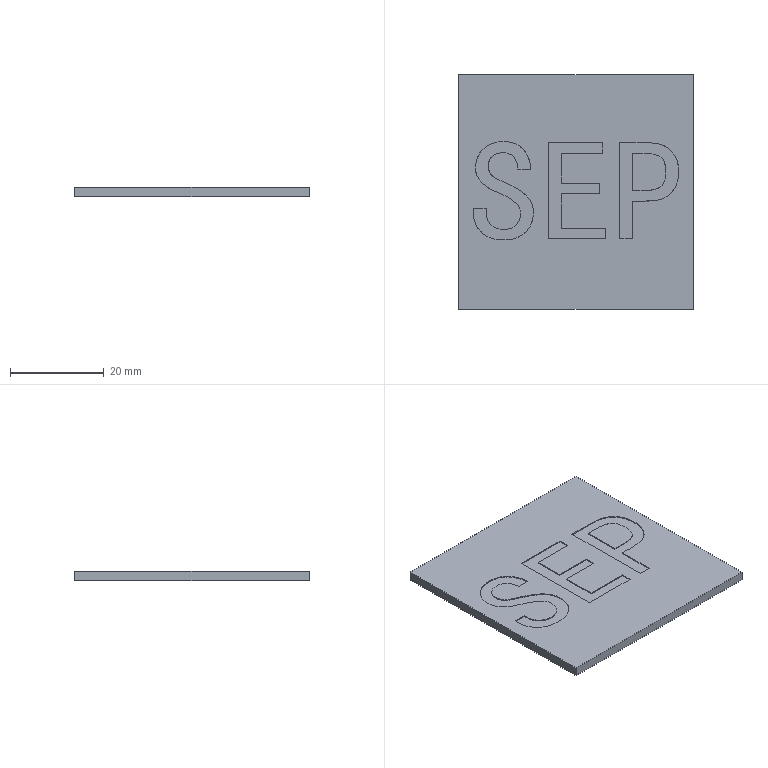Part | STEP file | lll_id1674_x_t | 1 solid | 38 faces | box 50 x 50 x 2 mm | volume 4930 mm3 | plane 28 | other 10
STEP:
#1=CARTESIAN_POINT('',(3913.931,-539.312,3.259));
#2=VERTEX_POINT('',#1);
#3=CARTESIAN_POINT('',(3918.013,-541.893,3.259));
#4=VERTEX_POINT('',#3);
#5=CARTESIAN_POINT('',(3913.931,-539.312,3.259));
#6=CARTESIAN_POINT('',(3915.691,-540.032,3.259));
#7=CARTESIAN_POINT('',(3917.052,-540.892,3.259));
#8=CARTESIAN_POINT('',(3918.013,-541.893,3.259));
#9=B_SPLINE_CURVE_WITH_KNOTS('',3,(#5,#6,#7,#8),.UNSPECIFIED.,.F.,.F.,(4,4),(0.,1.),.UNSPECIFIED.);
#10=EDGE_CURVE('',#2,#4,#9,.T.);
#11=ORIENTED_EDGE('',*,*,#10,.T.);
#12=CARTESIAN_POINT('',(3906.615,-544.587,3.259));
#13=VERTEX_POINT('',#12);
#14=CARTESIAN_POINT('',(3918.013,-541.893,3.259));
#15=CARTESIAN_POINT('',(3918.969,-542.888,3.259));
#16=CARTESIAN_POINT('',(3919.453,-544.03,3.259));
#17=CARTESIAN_POINT('',(3919.453,-547.151,3.259));
#18=CARTESIAN_POINT('',(3918.868,-548.607,3.259));
#19=CARTESIAN_POINT('',(3916.551,-550.767,3.259));
#20=CARTESIAN_POINT('',(3914.971,-551.307,3.259));
#21=CARTESIAN_POINT('',(3910.973,-551.307,3.259));
#22=CARTESIAN_POINT('',(3909.415,-550.75,3.259));
#23=CARTESIAN_POINT('',(3907.18,-548.503,3.259));
#24=CARTESIAN_POINT('',(3906.615,-547.112,3.259));
#25=CARTESIAN_POINT('',(3906.615,-545.149,3.259));
#26=CARTESIAN_POINT('',(3906.615,-544.868,3.259));
#27=CARTESIAN_POINT('',(3906.615,-544.587,3.259));
#28=B_SPLINE_CURVE_WITH_KNOTS('',3,(#14,#15,#16,#17,#18,#19,#20,#21,#22,#23,#24,#25,#26,#27),.UNSPECIFIED.,.F.,.F.,(4,2,2,2,2,2,4),(0.,0.1423,0.348,0.5536,0.7599,0.9656,1.),.UNSPECIFIED.);
#29=EDGE_CURVE('',#4,#13,#28,.T.);
#30=ORIENTED_EDGE('',*,*,#29,.T.);
#31=CARTESIAN_POINT('',(3909.376,-544.587,3.259));
#32=VERTEX_POINT('',#31);
#33=CARTESIAN_POINT('',(3907.995,-544.587,3.259));
#34=DIRECTION('',(1.,0.,0.));
#35=VECTOR('',#34,1.);
#36=LINE('',#33,#35);
#37=EDGE_CURVE('',#13,#32,#36,.T.);
#38=ORIENTED_EDGE('',*,*,#37,.T.);
#39=CARTESIAN_POINT('',(3912.491,-541.471,3.259));
#40=VERTEX_POINT('',#39);
#41=CARTESIAN_POINT('',(3909.376,-544.587,3.259));
#42=CARTESIAN_POINT('',(3909.376,-544.827,3.259));
#43=CARTESIAN_POINT('',(3909.376,-545.067,3.259));
#44=CARTESIAN_POINT('',(3909.376,-546.51,3.259));
#45=CARTESIAN_POINT('',(3909.736,-547.427,3.259));
#46=CARTESIAN_POINT('',(3911.175,-548.709,3.259));
#47=CARTESIAN_POINT('',(3912.013,-549.029,3.259));
#48=CARTESIAN_POINT('',(3914.251,-549.029,3.259));
#49=CARTESIAN_POINT('',(3915.19,-548.686,3.259));
#50=CARTESIAN_POINT('',(3916.391,-547.328,3.259));
#51=CARTESIAN_POINT('',(3916.692,-546.51,3.259));
#52=CARTESIAN_POINT('',(3916.692,-544.75,3.259));
#53=CARTESIAN_POINT('',(3916.332,-544.008,3.259));
#54=CARTESIAN_POINT('',(3914.889,-542.655,3.259));
#55=CARTESIAN_POINT('',(3913.852,-542.028,3.259));
#56=CARTESIAN_POINT('',(3912.491,-541.471,3.259));
#57=B_SPLINE_CURVE_WITH_KNOTS('',3,(#41,#42,#43,#44,#45,#46,#47,#48,#49,#50,#51,#52,#53,#54,#55,#56),.UNSPECIFIED.,.F.,.F.,(4,2,2,2,2,2,2,4),(0.,0.02829,0.1702,0.3121,0.5005,0.688,0.8437,1.),.UNSPECIFIED.);
#58=EDGE_CURVE('',#32,#40,#57,.T.);
#59=ORIENTED_EDGE('',*,*,#58,.T.);
#60=CARTESIAN_POINT('',(3918.851,-536.191,3.259));
#61=VERTEX_POINT('',#60);
#62=CARTESIAN_POINT('',(3912.491,-541.471,3.259));
#63=CARTESIAN_POINT('',(3910.573,-540.752,3.259));
#64=CARTESIAN_POINT('',(3909.196,-539.953,3.259));
#65=CARTESIAN_POINT('',(3907.514,-538.193,3.259));
#66=CARTESIAN_POINT('',(3907.092,-537.152,3.259));
#67=CARTESIAN_POINT('',(3907.092,-534.273,3.259));
#68=CARTESIAN_POINT('',(3907.672,-532.912,3.259));
#69=CARTESIAN_POINT('',(3909.997,-530.835,3.259));
#70=CARTESIAN_POINT('',(3911.372,-530.314,3.259));
#71=CARTESIAN_POINT('',(3915.05,-530.314,3.259));
#72=CARTESIAN_POINT('',(3916.551,-530.933,3.259));
#73=CARTESIAN_POINT('',(3918.391,-533.412,3.259));
#74=CARTESIAN_POINT('',(3918.851,-534.751,3.259));
#75=CARTESIAN_POINT('',(3918.851,-536.191,3.259));
#76=B_SPLINE_CURVE_WITH_KNOTS('',3,(#62,#63,#64,#65,#66,#67,#68,#69,#70,#71,#72,#73,#74,#75),.UNSPECIFIED.,.F.,.F.,(4,2,2,2,2,2,4),(0.,0.1195,0.2381,0.4047,0.5709,0.786,1.),.UNSPECIFIED.);
#77=EDGE_CURVE('',#40,#61,#76,.T.);
#78=ORIENTED_EDGE('',*,*,#77,.T.);
#79=CARTESIAN_POINT('',(3916.09,-536.191,3.259));
#80=VERTEX_POINT('',#79);
#81=CARTESIAN_POINT('',(3917.471,-536.191,3.259));
#82=DIRECTION('',(-1.,0.,0.));
#83=VECTOR('',#82,1.);
#84=LINE('',#81,#83);
#85=EDGE_CURVE('',#61,#80,#84,.T.);
#86=ORIENTED_EDGE('',*,*,#85,.T.);
#87=CARTESIAN_POINT('',(3910.692,-533.492,3.259));
#88=VERTEX_POINT('',#87);
#89=CARTESIAN_POINT('',(3916.09,-536.191,3.259));
#90=CARTESIAN_POINT('',(3916.169,-535.314,3.259));
#91=CARTESIAN_POINT('',(3915.933,-534.515,3.259));
#92=CARTESIAN_POINT('',(3914.81,-533.078,3.259));
#93=CARTESIAN_POINT('',(3914.009,-532.716,3.259));
#94=CARTESIAN_POINT('',(3912.013,-532.716,3.259));
#95=CARTESIAN_POINT('',(3911.254,-532.974,3.259));
#96=CARTESIAN_POINT('',(3910.692,-533.492,3.259));
#97=B_SPLINE_CURVE_WITH_KNOTS('',3,(#89,#90,#91,#92,#93,#94,#95,#96),.UNSPECIFIED.,.F.,.F.,(4,2,2,4),(0.,0.3422,0.6832,1.),.UNSPECIFIED.);
#98=EDGE_CURVE('',#80,#88,#97,.T.);
#99=ORIENTED_EDGE('',*,*,#98,.T.);
#100=CARTESIAN_POINT('',(3910.692,-533.492,3.259));
#101=CARTESIAN_POINT('',(3910.135,-534.015,3.259));
#102=CARTESIAN_POINT('',(3909.854,-534.712,3.259));
#103=CARTESIAN_POINT('',(3909.854,-536.315,3.259));
#104=CARTESIAN_POINT('',(3910.073,-536.933,3.259));
#105=CARTESIAN_POINT('',(3910.955,-537.974,3.259));
#106=CARTESIAN_POINT('',(3912.092,-538.592,3.259));
#107=CARTESIAN_POINT('',(3913.931,-539.312,3.259));
#108=B_SPLINE_CURVE_WITH_KNOTS('',3,(#100,#101,#102,#103,#104,#105,#106,#107),.UNSPECIFIED.,.F.,.F.,(4,2,2,4),(0.,0.3788,0.6876,1.),.UNSPECIFIED.);
#109=EDGE_CURVE('',#88,#2,#108,.T.);
#110=ORIENTED_EDGE('',*,*,#109,.T.);
#111=EDGE_LOOP('',(#11,#30,#38,#59,#78,#86,#99,#110));
#112=FACE_BOUND('',#111,.T.);
#113=CARTESIAN_POINT('',(3953.509,-566.065,3.259));
#114=VERTEX_POINT('',#113);
#115=CARTESIAN_POINT('',(3903.509,-566.065,3.259));
#116=VERTEX_POINT('',#115);
#117=CARTESIAN_POINT('',(4003.509,-566.065,3.259));
#118=DIRECTION('',(-1.,0.,0.));
#119=VECTOR('',#118,1.);
#120=LINE('',#117,#119);
#121=EDGE_CURVE('',#114,#116,#120,.T.);
#122=ORIENTED_EDGE('',*,*,#121,.F.);
#123=CARTESIAN_POINT('',(3953.509,-516.065,3.259));
#124=VERTEX_POINT('',#123);
#125=CARTESIAN_POINT('',(3953.509,-466.065,3.259));
#126=DIRECTION('',(0.,-1.,0.));
#127=VECTOR('',#126,1.);
#128=LINE('',#125,#127);
#129=EDGE_CURVE('',#124,#114,#128,.T.);
#130=ORIENTED_EDGE('',*,*,#129,.F.);
#131=CARTESIAN_POINT('',(3903.509,-516.065,3.259));
#132=VERTEX_POINT('',#131);
#133=CARTESIAN_POINT('',(4003.509,-516.065,3.259));
#134=DIRECTION('',(-1.,0.,0.));
#135=VECTOR('',#134,1.);
#136=LINE('',#133,#135);
#137=EDGE_CURVE('',#124,#132,#136,.T.);
#138=ORIENTED_EDGE('',*,*,#137,.T.);
#139=CARTESIAN_POINT('',(3903.509,-466.065,3.259));
#140=DIRECTION('',(0.,1.,0.));
#141=VECTOR('',#140,1.);
#142=LINE('',#139,#141);
#143=EDGE_CURVE('',#116,#132,#142,.T.);
#144=ORIENTED_EDGE('',*,*,#143,.F.);
#145=EDGE_LOOP('',(#122,#130,#138,#144));
#146=FACE_BOUND('',#145,.T.);
#147=CARTESIAN_POINT('',(3925.329,-548.787,3.259));
#148=VERTEX_POINT('',#147);
#149=CARTESIAN_POINT('',(3934.811,-548.787,3.259));
#150=VERTEX_POINT('',#149);
#151=CARTESIAN_POINT('',(3930.07,-548.787,3.259));
#152=DIRECTION('',(1.,0.,0.));
#153=VECTOR('',#152,1.);
#154=LINE('',#151,#153);
#155=EDGE_CURVE('',#148,#150,#154,.T.);
#156=ORIENTED_EDGE('',*,*,#155,.T.);
#157=CARTESIAN_POINT('',(3934.811,-551.065,3.259));
#158=VERTEX_POINT('',#157);
#159=CARTESIAN_POINT('',(3934.811,-549.926,3.259));
#160=DIRECTION('',(0.,-1.,0.));
#161=VECTOR('',#160,1.);
#162=LINE('',#159,#161);
#163=EDGE_CURVE('',#150,#158,#162,.T.);
#164=ORIENTED_EDGE('',*,*,#163,.T.);
#165=CARTESIAN_POINT('',(3922.574,-551.065,3.259));
#166=VERTEX_POINT('',#165);
#167=CARTESIAN_POINT('',(3928.692,-551.065,3.259));
#168=DIRECTION('',(-1.,0.,0.));
#169=VECTOR('',#168,1.);
#170=LINE('',#167,#169);
#171=EDGE_CURVE('',#158,#166,#170,.T.);
#172=ORIENTED_EDGE('',*,*,#171,.T.);
#173=CARTESIAN_POINT('',(3922.574,-530.556,3.259));
#174=VERTEX_POINT('',#173);
#175=CARTESIAN_POINT('',(3922.574,-540.811,3.259));
#176=DIRECTION('',(0.,1.,0.));
#177=VECTOR('',#176,1.);
#178=LINE('',#175,#177);
#179=EDGE_CURVE('',#166,#174,#178,.T.);
#180=ORIENTED_EDGE('',*,*,#179,.T.);
#181=CARTESIAN_POINT('',(3934.209,-530.556,3.259));
#182=VERTEX_POINT('',#181);
#183=CARTESIAN_POINT('',(3928.391,-530.556,3.259));
#184=DIRECTION('',(1.,0.,0.));
#185=VECTOR('',#184,1.);
#186=LINE('',#183,#185);
#187=EDGE_CURVE('',#174,#182,#186,.T.);
#188=ORIENTED_EDGE('',*,*,#187,.T.);
#189=CARTESIAN_POINT('',(3934.209,-532.834,3.259));
#190=VERTEX_POINT('',#189);
#191=CARTESIAN_POINT('',(3934.209,-531.695,3.259));
#192=DIRECTION('',(0.,-1.,0.));
#193=VECTOR('',#192,1.);
#194=LINE('',#191,#193);
#195=EDGE_CURVE('',#182,#190,#194,.T.);
#196=ORIENTED_EDGE('',*,*,#195,.T.);
#197=CARTESIAN_POINT('',(3925.329,-532.834,3.259));
#198=VERTEX_POINT('',#197);
#199=CARTESIAN_POINT('',(3929.769,-532.834,3.259));
#200=DIRECTION('',(-1.,0.,0.));
#201=VECTOR('',#200,1.);
#202=LINE('',#199,#201);
#203=EDGE_CURVE('',#190,#198,#202,.T.);
#204=ORIENTED_EDGE('',*,*,#203,.T.);
#205=CARTESIAN_POINT('',(3925.329,-539.194,3.259));
#206=VERTEX_POINT('',#205);
#207=CARTESIAN_POINT('',(3925.329,-536.014,3.259));
#208=DIRECTION('',(0.,-1.,0.));
#209=VECTOR('',#208,1.);
#210=LINE('',#207,#209);
#211=EDGE_CURVE('',#198,#206,#210,.T.);
#212=ORIENTED_EDGE('',*,*,#211,.T.);
#213=CARTESIAN_POINT('',(3933.489,-539.194,3.259));
#214=VERTEX_POINT('',#213);
#215=CARTESIAN_POINT('',(3929.409,-539.194,3.259));
#216=DIRECTION('',(1.,0.,0.));
#217=VECTOR('',#216,1.);
#218=LINE('',#215,#217);
#219=EDGE_CURVE('',#206,#214,#218,.T.);
#220=ORIENTED_EDGE('',*,*,#219,.T.);
#221=CARTESIAN_POINT('',(3933.489,-541.471,3.259));
#222=VERTEX_POINT('',#221);
#223=CARTESIAN_POINT('',(3933.489,-540.333,3.259));
#224=DIRECTION('',(0.,-1.,0.));
#225=VECTOR('',#224,1.);
#226=LINE('',#223,#225);
#227=EDGE_CURVE('',#214,#222,#226,.T.);
#228=ORIENTED_EDGE('',*,*,#227,.T.);
#229=CARTESIAN_POINT('',(3925.329,-541.471,3.259));
#230=VERTEX_POINT('',#229);
#231=CARTESIAN_POINT('',(3929.409,-541.471,3.259));
#232=DIRECTION('',(-1.,0.,0.));
#233=VECTOR('',#232,1.);
#234=LINE('',#231,#233);
#235=EDGE_CURVE('',#222,#230,#234,.T.);
#236=ORIENTED_EDGE('',*,*,#235,.T.);
#237=CARTESIAN_POINT('',(3925.329,-545.129,3.259));
#238=DIRECTION('',(0.,-1.,0.));
#239=VECTOR('',#238,1.);
#240=LINE('',#237,#239);
#241=EDGE_CURVE('',#230,#148,#240,.T.);
#242=ORIENTED_EDGE('',*,*,#241,.T.);
#243=EDGE_LOOP('',(#156,#164,#172,#180,#188,#196,#204,#212,#220,#228,#236,#242));
#244=FACE_BOUND('',#243,.T.);
#245=CARTESIAN_POINT('',(3937.808,-530.556,3.259));
#246=VERTEX_POINT('',#245);
#247=CARTESIAN_POINT('',(3948.729,-532.232,3.259));
#248=VERTEX_POINT('',#247);
#249=CARTESIAN_POINT('',(3937.808,-530.556,3.259));
#250=CARTESIAN_POINT('',(3939.889,-530.556,3.259));
#251=CARTESIAN_POINT('',(3941.969,-530.556,3.259));
#252=CARTESIAN_POINT('',(3946.046,-530.556,3.259));
#253=CARTESIAN_POINT('',(3947.604,-531.113,3.259));
#254=CARTESIAN_POINT('',(3948.729,-532.232,3.259));
#255=B_SPLINE_CURVE_WITH_KNOTS('',3,(#249,#250,#251,#252,#253,#254),.UNSPECIFIED.,.F.,.F.,(4,2,4),(0.,0.5103,1.),.UNSPECIFIED.);
#256=EDGE_CURVE('',#246,#248,#255,.T.);
#257=ORIENTED_EDGE('',*,*,#256,.T.);
#258=CARTESIAN_POINT('',(3940.569,-543.029,3.259));
#259=VERTEX_POINT('',#258);
#260=CARTESIAN_POINT('',(3948.729,-532.232,3.259));
#261=CARTESIAN_POINT('',(3949.848,-533.351,3.259));
#262=CARTESIAN_POINT('',(3950.404,-534.875,3.259));
#263=CARTESIAN_POINT('',(3950.404,-538.71,3.259));
#264=CARTESIAN_POINT('',(3949.848,-540.229,3.259));
#265=CARTESIAN_POINT('',(3947.61,-542.478,3.259));
#266=CARTESIAN_POINT('',(3946.046,-543.029,3.259));
#267=CARTESIAN_POINT('',(3942.89,-543.029,3.259));
#268=CARTESIAN_POINT('',(3941.729,-543.029,3.259));
#269=CARTESIAN_POINT('',(3940.569,-543.029,3.259));
#270=B_SPLINE_CURVE_WITH_KNOTS('',3,(#260,#261,#262,#263,#264,#265,#266,#267,#268,#269),.UNSPECIFIED.,.F.,.F.,(4,2,2,2,4),(0.,0.2792,0.5585,0.8377,1.),.UNSPECIFIED.);
#271=EDGE_CURVE('',#248,#259,#270,.T.);
#272=ORIENTED_EDGE('',*,*,#271,.T.);
#273=CARTESIAN_POINT('',(3940.569,-551.065,3.259));
#274=VERTEX_POINT('',#273);
#275=CARTESIAN_POINT('',(3940.569,-547.047,3.259));
#276=DIRECTION('',(0.,-1.,0.));
#277=VECTOR('',#276,1.);
#278=LINE('',#275,#277);
#279=EDGE_CURVE('',#259,#274,#278,.T.);
#280=ORIENTED_EDGE('',*,*,#279,.T.);
#281=CARTESIAN_POINT('',(3937.808,-551.065,3.259));
#282=VERTEX_POINT('',#281);
#283=CARTESIAN_POINT('',(3939.188,-551.065,3.259));
#284=DIRECTION('',(-1.,0.,0.));
#285=VECTOR('',#284,1.);
#286=LINE('',#283,#285);
#287=EDGE_CURVE('',#274,#282,#286,.T.);
#288=ORIENTED_EDGE('',*,*,#287,.T.);
#289=CARTESIAN_POINT('',(3937.808,-540.811,3.259));
#290=DIRECTION('',(0.,1.,0.));
#291=VECTOR('',#290,1.);
#292=LINE('',#289,#291);
#293=EDGE_CURVE('',#282,#246,#292,.T.);
#294=ORIENTED_EDGE('',*,*,#293,.T.);
#295=EDGE_LOOP('',(#257,#272,#280,#288,#294));
#296=FACE_BOUND('',#295,.T.);
#297=CARTESIAN_POINT('',(4003.509,-466.065,3.259));
#298=DIRECTION('',(0.,0.,1.));
#299=DIRECTION('',(1.,0.,0.));
#300=AXIS2_PLACEMENT_3D('',#297,#298,#299);
#301=PLANE('',#300);
#302=ADVANCED_FACE('',(#112,#146,#244,#296),#301,.T.);
#303=CARTESIAN_POINT('',(3953.509,-566.065,1.259));
#304=VERTEX_POINT('',#303);
#305=CARTESIAN_POINT('',(3953.509,-566.065,179.534));
#306=DIRECTION('',(0.,0.,1.));
#307=VECTOR('',#306,1.);
#308=LINE('',#305,#307);
#309=EDGE_CURVE('',#304,#114,#308,.T.);
#310=ORIENTED_EDGE('',*,*,#309,.F.);
#311=CARTESIAN_POINT('',(3953.509,-516.065,1.259));
#312=VERTEX_POINT('',#311);
#313=CARTESIAN_POINT('',(3953.509,-466.065,1.259));
#314=DIRECTION('',(0.,-1.,0.));
#315=VECTOR('',#314,1.);
#316=LINE('',#313,#315);
#317=EDGE_CURVE('',#312,#304,#316,.T.);
#318=ORIENTED_EDGE('',*,*,#317,.F.);
#319=CARTESIAN_POINT('',(3953.509,-516.065,2.109));
#320=DIRECTION('',(0.,0.,-1.));
#321=VECTOR('',#320,1.);
#322=LINE('',#319,#321);
#323=EDGE_CURVE('',#124,#312,#322,.T.);
#324=ORIENTED_EDGE('',*,*,#323,.F.);
#325=ORIENTED_EDGE('',*,*,#129,.T.);
#326=EDGE_LOOP('',(#310,#318,#324,#325));
#327=FACE_OUTER_BOUND('',#326,.T.);
#328=CARTESIAN_POINT('',(3953.509,-541.065,2.259));
#329=DIRECTION('',(1.,0.,0.));
#330=DIRECTION('',(0.,0.,-1.));
#331=AXIS2_PLACEMENT_3D('',#328,#329,#330);
#332=PLANE('',#331);
#333=ADVANCED_FACE('',(#327),#332,.T.);
#334=CARTESIAN_POINT('',(3903.509,-516.065,1.259));
#335=VERTEX_POINT('',#334);
#336=CARTESIAN_POINT('',(3903.509,-516.065,2.109));
#337=DIRECTION('',(0.,0.,1.));
#338=VECTOR('',#337,1.);
#339=LINE('',#336,#338);
#340=EDGE_CURVE('',#335,#132,#339,.T.);
#341=ORIENTED_EDGE('',*,*,#340,.F.);
#342=CARTESIAN_POINT('',(3903.509,-566.065,1.259));
#343=VERTEX_POINT('',#342);
#344=CARTESIAN_POINT('',(3903.509,-466.065,1.259));
#345=DIRECTION('',(0.,-1.,0.));
#346=VECTOR('',#345,1.);
#347=LINE('',#344,#346);
#348=EDGE_CURVE('',#335,#343,#347,.T.);
#349=ORIENTED_EDGE('',*,*,#348,.T.);
#350=CARTESIAN_POINT('',(3903.509,-566.065,179.534));
#351=DIRECTION('',(0.,0.,1.));
#352=VECTOR('',#351,1.);
#353=LINE('',#350,#352);
#354=EDGE_CURVE('',#343,#116,#353,.T.);
#355=ORIENTED_EDGE('',*,*,#354,.T.);
#356=ORIENTED_EDGE('',*,*,#143,.T.);
#357=EDGE_LOOP('',(#341,#349,#355,#356));
#358=FACE_OUTER_BOUND('',#357,.T.);
#359=CARTESIAN_POINT('',(3903.509,-516.065,2.109));
#360=DIRECTION('',(1.,0.,0.));
#361=DIRECTION('',(0.,0.,-1.));
#362=AXIS2_PLACEMENT_3D('',#359,#360,#361);
#363=PLANE('',#362);
#364=ADVANCED_FACE('',(#358),#363,.F.);
#365=ORIENTED_EDGE('',*,*,#137,.F.);
#366=ORIENTED_EDGE('',*,*,#323,.T.);
#367=CARTESIAN_POINT('',(2443.509,-516.065,1.259));
#368=DIRECTION('',(1.,0.,0.));
#369=VECTOR('',#368,1.);
#370=LINE('',#367,#369);
#371=EDGE_CURVE('',#335,#312,#370,.T.);
#372=ORIENTED_EDGE('',*,*,#371,.F.);
#373=ORIENTED_EDGE('',*,*,#340,.T.);
#374=EDGE_LOOP('',(#365,#366,#372,#373));
#375=FACE_OUTER_BOUND('',#374,.T.);
#376=CARTESIAN_POINT('',(3953.509,-516.065,2.109));
#377=DIRECTION('',(0.,1.,0.));
#378=DIRECTION('',(0.,0.,1.));
#379=AXIS2_PLACEMENT_3D('',#376,#377,#378);
#380=PLANE('',#379);
#381=ADVANCED_FACE('',(#375),#380,.T.);
#382=CARTESIAN_POINT('',(-3312.62,-566.065,1.259));
#383=DIRECTION('',(1.,0.,0.));
#384=VECTOR('',#383,1.);
#385=LINE('',#382,#384);
#386=EDGE_CURVE('',#343,#304,#385,.T.);
#387=ORIENTED_EDGE('',*,*,#386,.T.);
#388=ORIENTED_EDGE('',*,*,#309,.T.);
#389=ORIENTED_EDGE('',*,*,#121,.T.);
#390=ORIENTED_EDGE('',*,*,#354,.F.);
#391=EDGE_LOOP('',(#387,#388,#389,#390));
#392=FACE_OUTER_BOUND('',#391,.T.);
#393=CARTESIAN_POINT('',(-3312.62,-566.065,179.534));
#394=DIRECTION('',(0.,-1.,0.));
#395=DIRECTION('',(0.,0.,-1.));
#396=AXIS2_PLACEMENT_3D('',#393,#394,#395);
#397=PLANE('',#396);
#398=ADVANCED_FACE('',(#392),#397,.T.);
#399=ORIENTED_EDGE('',*,*,#371,.T.);
#400=ORIENTED_EDGE('',*,*,#317,.T.);
#401=ORIENTED_EDGE('',*,*,#386,.F.);
#402=ORIENTED_EDGE('',*,*,#348,.F.);
#403=EDGE_LOOP('',(#399,#400,#401,#402));
#404=FACE_OUTER_BOUND('',#403,.T.);
#405=CARTESIAN_POINT('',(2443.509,-466.065,1.259));
#406=DIRECTION('',(0.,0.,-1.));
#407=DIRECTION('',(-1.,0.,0.));
#408=AXIS2_PLACEMENT_3D('',#405,#406,#407);
#409=PLANE('',#408);
#410=ADVANCED_FACE('',(#404),#409,.T.);
#411=ORIENTED_EDGE('',*,*,#163,.F.);
#412=CARTESIAN_POINT('',(3934.811,-548.787,3.059));
#413=VERTEX_POINT('',#412);
#414=CARTESIAN_POINT('',(3934.811,-548.787,3.059));
#415=DIRECTION('',(0.,0.,-1.));
#416=VECTOR('',#415,1.);
#417=LINE('',#414,#416);
#418=EDGE_CURVE('',#150,#413,#417,.T.);
#419=ORIENTED_EDGE('',*,*,#418,.T.);
#420=CARTESIAN_POINT('',(3934.811,-551.065,3.059));
#421=VERTEX_POINT('',#420);
#422=CARTESIAN_POINT('',(3934.811,-549.926,3.059));
#423=DIRECTION('',(0.,1.,0.));
#424=VECTOR('',#423,1.);
#425=LINE('',#422,#424);
#426=EDGE_CURVE('',#421,#413,#425,.T.);
#427=ORIENTED_EDGE('',*,*,#426,.F.);
#428=CARTESIAN_POINT('',(3934.811,-551.065,3.059));
#429=DIRECTION('',(0.,0.,-1.));
#430=VECTOR('',#429,1.);
#431=LINE('',#428,#430);
#432=EDGE_CURVE('',#158,#421,#431,.T.);
#433=ORIENTED_EDGE('',*,*,#432,.F.);
#434=EDGE_LOOP('',(#411,#419,#427,#433));
#435=FACE_OUTER_BOUND('',#434,.T.);
#436=CARTESIAN_POINT('',(3934.811,-548.787,3.059));
#437=DIRECTION('',(-1.,0.,0.));
#438=DIRECTION('',(0.,0.,1.));
#439=AXIS2_PLACEMENT_3D('',#436,#437,#438);
#440=PLANE('',#439);
#441=ADVANCED_FACE('',(#435),#440,.T.);
#442=ORIENTED_EDGE('',*,*,#171,.F.);
#443=ORIENTED_EDGE('',*,*,#432,.T.);
#444=CARTESIAN_POINT('',(3922.574,-551.065,3.059));
#445=VERTEX_POINT('',#444);
#446=CARTESIAN_POINT('',(3928.692,-551.065,3.059));
#447=DIRECTION('',(1.,0.,0.));
#448=VECTOR('',#447,1.);
#449=LINE('',#446,#448);
#450=EDGE_CURVE('',#445,#421,#449,.T.);
#451=ORIENTED_EDGE('',*,*,#450,.F.);
#452=CARTESIAN_POINT('',(3922.574,-551.065,3.059));
#453=DIRECTION('',(0.,0.,-1.));
#454=VECTOR('',#453,1.);
#455=LINE('',#452,#454);
#456=EDGE_CURVE('',#166,#445,#455,.T.);
#457=ORIENTED_EDGE('',*,*,#456,.F.);
#458=EDGE_LOOP('',(#442,#443,#451,#457));
#459=FACE_OUTER_BOUND('',#458,.T.);
#460=CARTESIAN_POINT('',(3934.811,-551.065,3.059));
#461=DIRECTION('',(0.,1.,0.));
#462=DIRECTION('',(0.,0.,1.));
#463=AXIS2_PLACEMENT_3D('',#460,#461,#462);
#464=PLANE('',#463);
#465=ADVANCED_FACE('',(#459),#464,.T.);
#466=ORIENTED_EDGE('',*,*,#179,.F.);
#467=ORIENTED_EDGE('',*,*,#456,.T.);
#468=CARTESIAN_POINT('',(3922.574,-530.556,3.059));
#469=VERTEX_POINT('',#468);
#470=CARTESIAN_POINT('',(3922.574,-540.811,3.059));
#471=DIRECTION('',(0.,-1.,0.));
#472=VECTOR('',#471,1.);
#473=LINE('',#470,#472);
#474=EDGE_CURVE('',#469,#445,#473,.T.);
#475=ORIENTED_EDGE('',*,*,#474,.F.);
#476=CARTESIAN_POINT('',(3922.574,-530.556,3.059));
#477=DIRECTION('',(0.,0.,-1.));
#478=VECTOR('',#477,1.);
#479=LINE('',#476,#478);
#480=EDGE_CURVE('',#174,#469,#479,.T.);
#481=ORIENTED_EDGE('',*,*,#480,.F.);
#482=EDGE_LOOP('',(#466,#467,#475,#481));
#483=FACE_OUTER_BOUND('',#482,.T.);
#484=CARTESIAN_POINT('',(3922.574,-551.065,3.059));
#485=DIRECTION('',(1.,0.,0.));
#486=DIRECTION('',(0.,0.,-1.));
#487=AXIS2_PLACEMENT_3D('',#484,#485,#486);
#488=PLANE('',#487);
#489=ADVANCED_FACE('',(#483),#488,.T.);
#490=ORIENTED_EDGE('',*,*,#187,.F.);
#491=ORIENTED_EDGE('',*,*,#480,.T.);
#492=CARTESIAN_POINT('',(3934.209,-530.556,3.059));
#493=VERTEX_POINT('',#492);
#494=CARTESIAN_POINT('',(3928.391,-530.556,3.059));
#495=DIRECTION('',(-1.,0.,0.));
#496=VECTOR('',#495,1.);
#497=LINE('',#494,#496);
#498=EDGE_CURVE('',#493,#469,#497,.T.);
#499=ORIENTED_EDGE('',*,*,#498,.F.);
#500=CARTESIAN_POINT('',(3934.209,-530.556,3.059));
#501=DIRECTION('',(0.,0.,-1.));
#502=VECTOR('',#501,1.);
#503=LINE('',#500,#502);
#504=EDGE_CURVE('',#182,#493,#503,.T.);
#505=ORIENTED_EDGE('',*,*,#504,.F.);
#506=EDGE_LOOP('',(#490,#491,#499,#505));
#507=FACE_OUTER_BOUND('',#506,.T.);
#508=CARTESIAN_POINT('',(3922.574,-530.556,3.059));
#509=DIRECTION('',(0.,-1.,0.));
#510=DIRECTION('',(0.,0.,-1.));
#511=AXIS2_PLACEMENT_3D('',#508,#509,#510);
#512=PLANE('',#511);
#513=ADVANCED_FACE('',(#507),#512,.T.);
#514=ORIENTED_EDGE('',*,*,#195,.F.);
#515=ORIENTED_EDGE('',*,*,#504,.T.);
#516=CARTESIAN_POINT('',(3934.209,-532.834,3.059));
#517=VERTEX_POINT('',#516);
#518=CARTESIAN_POINT('',(3934.209,-531.695,3.059));
#519=DIRECTION('',(0.,1.,0.));
#520=VECTOR('',#519,1.);
#521=LINE('',#518,#520);
#522=EDGE_CURVE('',#517,#493,#521,.T.);
#523=ORIENTED_EDGE('',*,*,#522,.F.);
#524=CARTESIAN_POINT('',(3934.209,-532.834,3.059));
#525=DIRECTION('',(0.,0.,-1.));
#526=VECTOR('',#525,1.);
#527=LINE('',#524,#526);
#528=EDGE_CURVE('',#190,#517,#527,.T.);
#529=ORIENTED_EDGE('',*,*,#528,.F.);
#530=EDGE_LOOP('',(#514,#515,#523,#529));
#531=FACE_OUTER_BOUND('',#530,.T.);
#532=CARTESIAN_POINT('',(3934.209,-530.556,3.059));
#533=DIRECTION('',(-1.,0.,0.));
#534=DIRECTION('',(0.,0.,1.));
#535=AXIS2_PLACEMENT_3D('',#532,#533,#534);
#536=PLANE('',#535);
#537=ADVANCED_FACE('',(#531),#536,.T.);
#538=ORIENTED_EDGE('',*,*,#203,.F.);
#539=ORIENTED_EDGE('',*,*,#528,.T.);
#540=CARTESIAN_POINT('',(3925.329,-532.834,3.059));
#541=VERTEX_POINT('',#540);
#542=CARTESIAN_POINT('',(3929.769,-532.834,3.059));
#543=DIRECTION('',(1.,0.,0.));
#544=VECTOR('',#543,1.);
#545=LINE('',#542,#544);
#546=EDGE_CURVE('',#541,#517,#545,.T.);
#547=ORIENTED_EDGE('',*,*,#546,.F.);
#548=CARTESIAN_POINT('',(3925.329,-532.834,3.059));
#549=DIRECTION('',(0.,0.,-1.));
#550=VECTOR('',#549,1.);
#551=LINE('',#548,#550);
#552=EDGE_CURVE('',#198,#541,#551,.T.);
#553=ORIENTED_EDGE('',*,*,#552,.F.);
#554=EDGE_LOOP('',(#538,#539,#547,#553));
#555=FACE_OUTER_BOUND('',#554,.T.);
#556=CARTESIAN_POINT('',(3934.209,-532.834,3.059));
#557=DIRECTION('',(0.,1.,0.));
#558=DIRECTION('',(0.,0.,1.));
#559=AXIS2_PLACEMENT_3D('',#556,#557,#558);
#560=PLANE('',#559);
#561=ADVANCED_FACE('',(#555),#560,.T.);
#562=ORIENTED_EDGE('',*,*,#211,.F.);
#563=ORIENTED_EDGE('',*,*,#552,.T.);
#564=CARTESIAN_POINT('',(3925.329,-539.194,3.059));
#565=VERTEX_POINT('',#564);
#566=CARTESIAN_POINT('',(3925.329,-536.014,3.059));
#567=DIRECTION('',(0.,1.,0.));
#568=VECTOR('',#567,1.);
#569=LINE('',#566,#568);
#570=EDGE_CURVE('',#565,#541,#569,.T.);
#571=ORIENTED_EDGE('',*,*,#570,.F.);
#572=CARTESIAN_POINT('',(3925.329,-539.194,3.059));
#573=DIRECTION('',(0.,0.,-1.));
#574=VECTOR('',#573,1.);
#575=LINE('',#572,#574);
#576=EDGE_CURVE('',#206,#565,#575,.T.);
#577=ORIENTED_EDGE('',*,*,#576,.F.);
#578=EDGE_LOOP('',(#562,#563,#571,#577));
#579=FACE_OUTER_BOUND('',#578,.T.);
#580=CARTESIAN_POINT('',(3925.329,-532.834,3.059));
#581=DIRECTION('',(-1.,0.,0.));
#582=DIRECTION('',(0.,0.,1.));
#583=AXIS2_PLACEMENT_3D('',#580,#581,#582);
#584=PLANE('',#583);
#585=ADVANCED_FACE('',(#579),#584,.T.);
#586=ORIENTED_EDGE('',*,*,#219,.F.);
#587=ORIENTED_EDGE('',*,*,#576,.T.);
#588=CARTESIAN_POINT('',(3933.489,-539.194,3.059));
#589=VERTEX_POINT('',#588);
#590=CARTESIAN_POINT('',(3929.409,-539.194,3.059));
#591=DIRECTION('',(-1.,0.,0.));
#592=VECTOR('',#591,1.);
#593=LINE('',#590,#592);
#594=EDGE_CURVE('',#589,#565,#593,.T.);
#595=ORIENTED_EDGE('',*,*,#594,.F.);
#596=CARTESIAN_POINT('',(3933.489,-539.194,3.059));
#597=DIRECTION('',(0.,0.,-1.));
#598=VECTOR('',#597,1.);
#599=LINE('',#596,#598);
#600=EDGE_CURVE('',#214,#589,#599,.T.);
#601=ORIENTED_EDGE('',*,*,#600,.F.);
#602=EDGE_LOOP('',(#586,#587,#595,#601));
#603=FACE_OUTER_BOUND('',#602,.T.);
#604=CARTESIAN_POINT('',(3925.329,-539.194,3.059));
#605=DIRECTION('',(0.,-1.,0.));
#606=DIRECTION('',(0.,0.,-1.));
#607=AXIS2_PLACEMENT_3D('',#604,#605,#606);
#608=PLANE('',#607);
#609=ADVANCED_FACE('',(#603),#608,.T.);
#610=ORIENTED_EDGE('',*,*,#227,.F.);
#611=ORIENTED_EDGE('',*,*,#600,.T.);
#612=CARTESIAN_POINT('',(3933.489,-541.471,3.059));
#613=VERTEX_POINT('',#612);
#614=CARTESIAN_POINT('',(3933.489,-540.333,3.059));
#615=DIRECTION('',(0.,1.,0.));
#616=VECTOR('',#615,1.);
#617=LINE('',#614,#616);
#618=EDGE_CURVE('',#613,#589,#617,.T.);
#619=ORIENTED_EDGE('',*,*,#618,.F.);
#620=CARTESIAN_POINT('',(3933.489,-541.471,3.059));
#621=DIRECTION('',(0.,0.,-1.));
#622=VECTOR('',#621,1.);
#623=LINE('',#620,#622);
#624=EDGE_CURVE('',#222,#613,#623,.T.);
#625=ORIENTED_EDGE('',*,*,#624,.F.);
#626=EDGE_LOOP('',(#610,#611,#619,#625));
#627=FACE_OUTER_BOUND('',#626,.T.);
#628=CARTESIAN_POINT('',(3933.489,-539.194,3.059));
#629=DIRECTION('',(-1.,0.,0.));
#630=DIRECTION('',(0.,0.,1.));
#631=AXIS2_PLACEMENT_3D('',#628,#629,#630);
#632=PLANE('',#631);
#633=ADVANCED_FACE('',(#627),#632,.T.);
#634=ORIENTED_EDGE('',*,*,#235,.F.);
#635=ORIENTED_EDGE('',*,*,#624,.T.);
#636=CARTESIAN_POINT('',(3925.329,-541.471,3.059));
#637=VERTEX_POINT('',#636);
#638=CARTESIAN_POINT('',(3929.409,-541.471,3.059));
#639=DIRECTION('',(1.,0.,0.));
#640=VECTOR('',#639,1.);
#641=LINE('',#638,#640);
#642=EDGE_CURVE('',#637,#613,#641,.T.);
#643=ORIENTED_EDGE('',*,*,#642,.F.);
#644=CARTESIAN_POINT('',(3925.329,-541.471,3.059));
#645=DIRECTION('',(0.,0.,-1.));
#646=VECTOR('',#645,1.);
#647=LINE('',#644,#646);
#648=EDGE_CURVE('',#230,#637,#647,.T.);
#649=ORIENTED_EDGE('',*,*,#648,.F.);
#650=EDGE_LOOP('',(#634,#635,#643,#649));
#651=FACE_OUTER_BOUND('',#650,.T.);
#652=CARTESIAN_POINT('',(3933.489,-541.471,3.059));
#653=DIRECTION('',(0.,1.,0.));
#654=DIRECTION('',(0.,0.,1.));
#655=AXIS2_PLACEMENT_3D('',#652,#653,#654);
#656=PLANE('',#655);
#657=ADVANCED_FACE('',(#651),#656,.T.);
#658=ORIENTED_EDGE('',*,*,#241,.F.);
#659=ORIENTED_EDGE('',*,*,#648,.T.);
#660=CARTESIAN_POINT('',(3925.329,-548.787,3.059));
#661=VERTEX_POINT('',#660);
#662=CARTESIAN_POINT('',(3925.329,-545.129,3.059));
#663=DIRECTION('',(0.,1.,0.));
#664=VECTOR('',#663,1.);
#665=LINE('',#662,#664);
#666=EDGE_CURVE('',#661,#637,#665,.T.);
#667=ORIENTED_EDGE('',*,*,#666,.F.);
#668=CARTESIAN_POINT('',(3925.329,-548.787,3.059));
#669=DIRECTION('',(0.,0.,-1.));
#670=VECTOR('',#669,1.);
#671=LINE('',#668,#670);
#672=EDGE_CURVE('',#148,#661,#671,.T.);
#673=ORIENTED_EDGE('',*,*,#672,.F.);
#674=EDGE_LOOP('',(#658,#659,#667,#673));
#675=FACE_OUTER_BOUND('',#674,.T.);
#676=CARTESIAN_POINT('',(3925.329,-541.471,3.059));
#677=DIRECTION('',(-1.,0.,0.));
#678=DIRECTION('',(0.,0.,1.));
#679=AXIS2_PLACEMENT_3D('',#676,#677,#678);
#680=PLANE('',#679);
#681=ADVANCED_FACE('',(#675),#680,.T.);
#682=ORIENTED_EDGE('',*,*,#155,.F.);
#683=ORIENTED_EDGE('',*,*,#672,.T.);
#684=CARTESIAN_POINT('',(3930.07,-548.787,3.059));
#685=DIRECTION('',(-1.,0.,0.));
#686=VECTOR('',#685,1.);
#687=LINE('',#684,#686);
#688=EDGE_CURVE('',#413,#661,#687,.T.);
#689=ORIENTED_EDGE('',*,*,#688,.F.);
#690=ORIENTED_EDGE('',*,*,#418,.F.);
#691=EDGE_LOOP('',(#682,#683,#689,#690));
#692=FACE_OUTER_BOUND('',#691,.T.);
#693=CARTESIAN_POINT('',(3925.329,-548.787,3.059));
#694=DIRECTION('',(0.,-1.,0.));
#695=DIRECTION('',(0.,0.,-1.));
#696=AXIS2_PLACEMENT_3D('',#693,#694,#695);
#697=PLANE('',#696);
#698=ADVANCED_FACE('',(#692),#697,.T.);
#699=ORIENTED_EDGE('',*,*,#426,.T.);
#700=ORIENTED_EDGE('',*,*,#688,.T.);
#701=ORIENTED_EDGE('',*,*,#666,.T.);
#702=ORIENTED_EDGE('',*,*,#642,.T.);
#703=ORIENTED_EDGE('',*,*,#618,.T.);
#704=ORIENTED_EDGE('',*,*,#594,.T.);
#705=ORIENTED_EDGE('',*,*,#570,.T.);
#706=ORIENTED_EDGE('',*,*,#546,.T.);
#707=ORIENTED_EDGE('',*,*,#522,.T.);
#708=ORIENTED_EDGE('',*,*,#498,.T.);
#709=ORIENTED_EDGE('',*,*,#474,.T.);
#710=ORIENTED_EDGE('',*,*,#450,.T.);
#711=EDGE_LOOP('',(#699,#700,#701,#702,#703,#704,#705,#706,#707,#708,#709,#710));
#712=FACE_OUTER_BOUND('',#711,.T.);
#713=CARTESIAN_POINT('',(3934.811,-549.926,3.059));
#714=DIRECTION('',(0.,0.,1.));
#715=DIRECTION('',(1.,0.,0.));
#716=AXIS2_PLACEMENT_3D('',#713,#714,#715);
#717=PLANE('',#716);
#718=ADVANCED_FACE('',(#712),#717,.T.);
#719=ORIENTED_EDGE('',*,*,#29,.F.);
#720=CARTESIAN_POINT('',(3918.013,-541.893,3.059));
#721=VERTEX_POINT('',#720);
#722=CARTESIAN_POINT('',(3918.013,-541.893,3.059));
#723=DIRECTION('',(0.,0.,-1.));
#724=VECTOR('',#723,1.);
#725=LINE('',#722,#724);
#726=EDGE_CURVE('',#4,#721,#725,.T.);
#727=ORIENTED_EDGE('',*,*,#726,.T.);
#728=CARTESIAN_POINT('',(3906.615,-544.587,3.059));
#729=VERTEX_POINT('',#728);
#730=CARTESIAN_POINT('',(3906.615,-544.587,3.059));
#731=CARTESIAN_POINT('',(3906.615,-544.868,3.059));
#732=CARTESIAN_POINT('',(3906.615,-545.149,3.059));
#733=CARTESIAN_POINT('',(3906.615,-547.112,3.059));
#734=CARTESIAN_POINT('',(3907.18,-548.503,3.059));
#735=CARTESIAN_POINT('',(3909.415,-550.75,3.059));
#736=CARTESIAN_POINT('',(3910.973,-551.307,3.059));
#737=CARTESIAN_POINT('',(3914.971,-551.307,3.059));
#738=CARTESIAN_POINT('',(3916.551,-550.767,3.059));
#739=CARTESIAN_POINT('',(3918.868,-548.607,3.059));
#740=CARTESIAN_POINT('',(3919.453,-547.151,3.059));
#741=CARTESIAN_POINT('',(3919.453,-544.03,3.059));
#742=CARTESIAN_POINT('',(3918.969,-542.888,3.059));
#743=CARTESIAN_POINT('',(3918.013,-541.893,3.059));
#744=B_SPLINE_CURVE_WITH_KNOTS('',3,(#730,#731,#732,#733,#734,#735,#736,#737,#738,#739,#740,#741,#742,#743),.UNSPECIFIED.,.F.,.F.,(4,2,2,2,2,2,4),(0.,0.0344,0.2401,0.4464,0.652,0.8577,1.),.UNSPECIFIED.);
#745=EDGE_CURVE('',#729,#721,#744,.T.);
#746=ORIENTED_EDGE('',*,*,#745,.F.);
#747=CARTESIAN_POINT('',(3906.615,-544.587,3.059));
#748=DIRECTION('',(0.,0.,-1.));
#749=VECTOR('',#748,1.);
#750=LINE('',#747,#749);
#751=EDGE_CURVE('',#13,#729,#750,.T.);
#752=ORIENTED_EDGE('',*,*,#751,.F.);
#753=EDGE_LOOP('',(#719,#727,#746,#752));
#754=FACE_OUTER_BOUND('',#753,.T.);
#755=CARTESIAN_POINT('',(3918.013,-541.893,3.059));
#756=CARTESIAN_POINT('',(3918.969,-542.888,3.059));
#757=CARTESIAN_POINT('',(3919.453,-544.03,3.059));
#758=CARTESIAN_POINT('',(3919.453,-547.151,3.059));
#759=CARTESIAN_POINT('',(3918.868,-548.607,3.059));
#760=CARTESIAN_POINT('',(3916.551,-550.767,3.059));
#761=CARTESIAN_POINT('',(3914.971,-551.307,3.059));
#762=CARTESIAN_POINT('',(3910.973,-551.307,3.059));
#763=CARTESIAN_POINT('',(3909.415,-550.75,3.059));
#764=CARTESIAN_POINT('',(3907.18,-548.503,3.059));
#765=CARTESIAN_POINT('',(3906.615,-547.112,3.059));
#766=CARTESIAN_POINT('',(3906.615,-545.149,3.059));
#767=CARTESIAN_POINT('',(3906.615,-544.868,3.059));
#768=CARTESIAN_POINT('',(3906.615,-544.587,3.059));
#769=B_SPLINE_CURVE_WITH_KNOTS('',3,(#755,#756,#757,#758,#759,#760,#761,#762,#763,#764,#765,#766,#767,#768),.UNSPECIFIED.,.F.,.F.,(4,2,2,2,2,2,4),(0.,0.1423,0.348,0.5536,0.7599,0.9656,1.),.UNSPECIFIED.);
#770=DIRECTION('',(0.,0.,1.));
#771=VECTOR('',#770,1.);
#772=SURFACE_OF_LINEAR_EXTRUSION('',#769,#771);
#773=ADVANCED_FACE('',(#754),#772,.T.);
#774=ORIENTED_EDGE('',*,*,#37,.F.);
#775=ORIENTED_EDGE('',*,*,#751,.T.);
#776=CARTESIAN_POINT('',(3909.376,-544.587,3.059));
#777=VERTEX_POINT('',#776);
#778=CARTESIAN_POINT('',(3907.995,-544.587,3.059));
#779=DIRECTION('',(-1.,0.,0.));
#780=VECTOR('',#779,1.);
#781=LINE('',#778,#780);
#782=EDGE_CURVE('',#777,#729,#781,.T.);
#783=ORIENTED_EDGE('',*,*,#782,.F.);
#784=CARTESIAN_POINT('',(3909.376,-544.587,3.059));
#785=DIRECTION('',(0.,0.,-1.));
#786=VECTOR('',#785,1.);
#787=LINE('',#784,#786);
#788=EDGE_CURVE('',#32,#777,#787,.T.);
#789=ORIENTED_EDGE('',*,*,#788,.F.);
#790=EDGE_LOOP('',(#774,#775,#783,#789));
#791=FACE_OUTER_BOUND('',#790,.T.);
#792=CARTESIAN_POINT('',(3906.615,-544.587,3.059));
#793=DIRECTION('',(0.,-1.,0.));
#794=DIRECTION('',(0.,0.,-1.));
#795=AXIS2_PLACEMENT_3D('',#792,#793,#794);
#796=PLANE('',#795);
#797=ADVANCED_FACE('',(#791),#796,.T.);
#798=ORIENTED_EDGE('',*,*,#58,.F.);
#799=ORIENTED_EDGE('',*,*,#788,.T.);
#800=CARTESIAN_POINT('',(3912.491,-541.471,3.059));
#801=VERTEX_POINT('',#800);
#802=CARTESIAN_POINT('',(3912.491,-541.471,3.059));
#803=CARTESIAN_POINT('',(3913.852,-542.028,3.059));
#804=CARTESIAN_POINT('',(3914.889,-542.655,3.059));
#805=CARTESIAN_POINT('',(3916.332,-544.008,3.059));
#806=CARTESIAN_POINT('',(3916.692,-544.75,3.059));
#807=CARTESIAN_POINT('',(3916.692,-546.51,3.059));
#808=CARTESIAN_POINT('',(3916.391,-547.328,3.059));
#809=CARTESIAN_POINT('',(3915.19,-548.686,3.059));
#810=CARTESIAN_POINT('',(3914.251,-549.029,3.059));
#811=CARTESIAN_POINT('',(3912.013,-549.029,3.059));
#812=CARTESIAN_POINT('',(3911.175,-548.709,3.059));
#813=CARTESIAN_POINT('',(3909.736,-547.427,3.059));
#814=CARTESIAN_POINT('',(3909.376,-546.51,3.059));
#815=CARTESIAN_POINT('',(3909.376,-545.067,3.059));
#816=CARTESIAN_POINT('',(3909.376,-544.827,3.059));
#817=CARTESIAN_POINT('',(3909.376,-544.587,3.059));
#818=B_SPLINE_CURVE_WITH_KNOTS('',3,(#802,#803,#804,#805,#806,#807,#808,#809,#810,#811,#812,#813,#814,#815,#816,#817),.UNSPECIFIED.,.F.,.F.,(4,2,2,2,2,2,2,4),(0.,0.1563,0.312,0.4995,0.6879,0.8298,0.9717,1.),.UNSPECIFIED.);
#819=EDGE_CURVE('',#801,#777,#818,.T.);
#820=ORIENTED_EDGE('',*,*,#819,.F.);
#821=CARTESIAN_POINT('',(3912.491,-541.471,3.059));
#822=DIRECTION('',(0.,0.,-1.));
#823=VECTOR('',#822,1.);
#824=LINE('',#821,#823);
#825=EDGE_CURVE('',#40,#801,#824,.T.);
#826=ORIENTED_EDGE('',*,*,#825,.F.);
#827=EDGE_LOOP('',(#798,#799,#820,#826));
#828=FACE_OUTER_BOUND('',#827,.T.);
#829=CARTESIAN_POINT('',(3909.376,-544.587,3.059));
#830=CARTESIAN_POINT('',(3909.376,-544.827,3.059));
#831=CARTESIAN_POINT('',(3909.376,-545.067,3.059));
#832=CARTESIAN_POINT('',(3909.376,-546.51,3.059));
#833=CARTESIAN_POINT('',(3909.736,-547.427,3.059));
#834=CARTESIAN_POINT('',(3911.175,-548.709,3.059));
#835=CARTESIAN_POINT('',(3912.013,-549.029,3.059));
#836=CARTESIAN_POINT('',(3914.251,-549.029,3.059));
#837=CARTESIAN_POINT('',(3915.19,-548.686,3.059));
#838=CARTESIAN_POINT('',(3916.391,-547.328,3.059));
#839=CARTESIAN_POINT('',(3916.692,-546.51,3.059));
#840=CARTESIAN_POINT('',(3916.692,-544.75,3.059));
#841=CARTESIAN_POINT('',(3916.332,-544.008,3.059));
#842=CARTESIAN_POINT('',(3914.889,-542.655,3.059));
#843=CARTESIAN_POINT('',(3913.852,-542.028,3.059));
#844=CARTESIAN_POINT('',(3912.491,-541.471,3.059));
#845=B_SPLINE_CURVE_WITH_KNOTS('',3,(#829,#830,#831,#832,#833,#834,#835,#836,#837,#838,#839,#840,#841,#842,#843,#844),.UNSPECIFIED.,.F.,.F.,(4,2,2,2,2,2,2,4),(0.,0.02829,0.1702,0.3121,0.5005,0.688,0.8437,1.),.UNSPECIFIED.);
#846=DIRECTION('',(0.,0.,1.));
#847=VECTOR('',#846,1.);
#848=SURFACE_OF_LINEAR_EXTRUSION('',#845,#847);
#849=ADVANCED_FACE('',(#828),#848,.T.);
#850=ORIENTED_EDGE('',*,*,#77,.F.);
#851=ORIENTED_EDGE('',*,*,#825,.T.);
#852=CARTESIAN_POINT('',(3918.851,-536.191,3.059));
#853=VERTEX_POINT('',#852);
#854=CARTESIAN_POINT('',(3918.851,-536.191,3.059));
#855=CARTESIAN_POINT('',(3918.851,-534.751,3.059));
#856=CARTESIAN_POINT('',(3918.391,-533.412,3.059));
#857=CARTESIAN_POINT('',(3916.551,-530.933,3.059));
#858=CARTESIAN_POINT('',(3915.05,-530.314,3.059));
#859=CARTESIAN_POINT('',(3911.372,-530.314,3.059));
#860=CARTESIAN_POINT('',(3909.997,-530.835,3.059));
#861=CARTESIAN_POINT('',(3907.672,-532.912,3.059));
#862=CARTESIAN_POINT('',(3907.092,-534.273,3.059));
#863=CARTESIAN_POINT('',(3907.092,-537.152,3.059));
#864=CARTESIAN_POINT('',(3907.514,-538.193,3.059));
#865=CARTESIAN_POINT('',(3909.196,-539.953,3.059));
#866=CARTESIAN_POINT('',(3910.573,-540.752,3.059));
#867=CARTESIAN_POINT('',(3912.491,-541.471,3.059));
#868=B_SPLINE_CURVE_WITH_KNOTS('',3,(#854,#855,#856,#857,#858,#859,#860,#861,#862,#863,#864,#865,#866,#867),.UNSPECIFIED.,.F.,.F.,(4,2,2,2,2,2,4),(0.,0.214,0.4291,0.5953,0.7619,0.8805,1.),.UNSPECIFIED.);
#869=EDGE_CURVE('',#853,#801,#868,.T.);
#870=ORIENTED_EDGE('',*,*,#869,.F.);
#871=CARTESIAN_POINT('',(3918.851,-536.191,3.059));
#872=DIRECTION('',(0.,0.,-1.));
#873=VECTOR('',#872,1.);
#874=LINE('',#871,#873);
#875=EDGE_CURVE('',#61,#853,#874,.T.);
#876=ORIENTED_EDGE('',*,*,#875,.F.);
#877=EDGE_LOOP('',(#850,#851,#870,#876));
#878=FACE_OUTER_BOUND('',#877,.T.);
#879=CARTESIAN_POINT('',(3912.491,-541.471,3.059));
#880=CARTESIAN_POINT('',(3910.573,-540.752,3.059));
#881=CARTESIAN_POINT('',(3909.196,-539.953,3.059));
#882=CARTESIAN_POINT('',(3907.514,-538.193,3.059));
#883=CARTESIAN_POINT('',(3907.092,-537.152,3.059));
#884=CARTESIAN_POINT('',(3907.092,-534.273,3.059));
#885=CARTESIAN_POINT('',(3907.672,-532.912,3.059));
#886=CARTESIAN_POINT('',(3909.997,-530.835,3.059));
#887=CARTESIAN_POINT('',(3911.372,-530.314,3.059));
#888=CARTESIAN_POINT('',(3915.05,-530.314,3.059));
#889=CARTESIAN_POINT('',(3916.551,-530.933,3.059));
#890=CARTESIAN_POINT('',(3918.391,-533.412,3.059));
#891=CARTESIAN_POINT('',(3918.851,-534.751,3.059));
#892=CARTESIAN_POINT('',(3918.851,-536.191,3.059));
#893=B_SPLINE_CURVE_WITH_KNOTS('',3,(#879,#880,#881,#882,#883,#884,#885,#886,#887,#888,#889,#890,#891,#892),.UNSPECIFIED.,.F.,.F.,(4,2,2,2,2,2,4),(0.,0.1195,0.2381,0.4047,0.5709,0.786,1.),.UNSPECIFIED.);
#894=DIRECTION('',(0.,0.,1.));
#895=VECTOR('',#894,1.);
#896=SURFACE_OF_LINEAR_EXTRUSION('',#893,#895);
#897=ADVANCED_FACE('',(#878),#896,.T.);
#898=ORIENTED_EDGE('',*,*,#85,.F.);
#899=ORIENTED_EDGE('',*,*,#875,.T.);
#900=CARTESIAN_POINT('',(3916.09,-536.191,3.059));
#901=VERTEX_POINT('',#900);
#902=CARTESIAN_POINT('',(3917.471,-536.191,3.059));
#903=DIRECTION('',(1.,0.,0.));
#904=VECTOR('',#903,1.);
#905=LINE('',#902,#904);
#906=EDGE_CURVE('',#901,#853,#905,.T.);
#907=ORIENTED_EDGE('',*,*,#906,.F.);
#908=CARTESIAN_POINT('',(3916.09,-536.191,3.059));
#909=DIRECTION('',(0.,0.,-1.));
#910=VECTOR('',#909,1.);
#911=LINE('',#908,#910);
#912=EDGE_CURVE('',#80,#901,#911,.T.);
#913=ORIENTED_EDGE('',*,*,#912,.F.);
#914=EDGE_LOOP('',(#898,#899,#907,#913));
#915=FACE_OUTER_BOUND('',#914,.T.);
#916=CARTESIAN_POINT('',(3918.851,-536.191,3.059));
#917=DIRECTION('',(0.,1.,0.));
#918=DIRECTION('',(0.,0.,1.));
#919=AXIS2_PLACEMENT_3D('',#916,#917,#918);
#920=PLANE('',#919);
#921=ADVANCED_FACE('',(#915),#920,.T.);
#922=ORIENTED_EDGE('',*,*,#98,.F.);
#923=ORIENTED_EDGE('',*,*,#912,.T.);
#924=CARTESIAN_POINT('',(3910.692,-533.492,3.059));
#925=VERTEX_POINT('',#924);
#926=CARTESIAN_POINT('',(3910.692,-533.492,3.059));
#927=CARTESIAN_POINT('',(3911.254,-532.974,3.059));
#928=CARTESIAN_POINT('',(3912.013,-532.716,3.059));
#929=CARTESIAN_POINT('',(3914.009,-532.716,3.059));
#930=CARTESIAN_POINT('',(3914.81,-533.078,3.059));
#931=CARTESIAN_POINT('',(3915.933,-534.515,3.059));
#932=CARTESIAN_POINT('',(3916.169,-535.314,3.059));
#933=CARTESIAN_POINT('',(3916.09,-536.191,3.059));
#934=B_SPLINE_CURVE_WITH_KNOTS('',3,(#926,#927,#928,#929,#930,#931,#932,#933),.UNSPECIFIED.,.F.,.F.,(4,2,2,4),(0.,0.3168,0.6578,1.),.UNSPECIFIED.);
#935=EDGE_CURVE('',#925,#901,#934,.T.);
#936=ORIENTED_EDGE('',*,*,#935,.F.);
#937=CARTESIAN_POINT('',(3910.692,-533.492,3.059));
#938=DIRECTION('',(0.,0.,-1.));
#939=VECTOR('',#938,1.);
#940=LINE('',#937,#939);
#941=EDGE_CURVE('',#88,#925,#940,.T.);
#942=ORIENTED_EDGE('',*,*,#941,.F.);
#943=EDGE_LOOP('',(#922,#923,#936,#942));
#944=FACE_OUTER_BOUND('',#943,.T.);
#945=CARTESIAN_POINT('',(3916.09,-536.191,3.059));
#946=CARTESIAN_POINT('',(3916.169,-535.314,3.059));
#947=CARTESIAN_POINT('',(3915.933,-534.515,3.059));
#948=CARTESIAN_POINT('',(3914.81,-533.078,3.059));
#949=CARTESIAN_POINT('',(3914.009,-532.716,3.059));
#950=CARTESIAN_POINT('',(3912.013,-532.716,3.059));
#951=CARTESIAN_POINT('',(3911.254,-532.974,3.059));
#952=CARTESIAN_POINT('',(3910.692,-533.492,3.059));
#953=B_SPLINE_CURVE_WITH_KNOTS('',3,(#945,#946,#947,#948,#949,#950,#951,#952),.UNSPECIFIED.,.F.,.F.,(4,2,2,4),(0.,0.3422,0.6832,1.),.UNSPECIFIED.);
#954=DIRECTION('',(0.,0.,1.));
#955=VECTOR('',#954,1.);
#956=SURFACE_OF_LINEAR_EXTRUSION('',#953,#955);
#957=ADVANCED_FACE('',(#944),#956,.T.);
#958=ORIENTED_EDGE('',*,*,#109,.F.);
#959=ORIENTED_EDGE('',*,*,#941,.T.);
#960=CARTESIAN_POINT('',(3913.931,-539.312,3.059));
#961=VERTEX_POINT('',#960);
#962=CARTESIAN_POINT('',(3913.931,-539.312,3.059));
#963=CARTESIAN_POINT('',(3912.092,-538.592,3.059));
#964=CARTESIAN_POINT('',(3910.955,-537.974,3.059));
#965=CARTESIAN_POINT('',(3910.073,-536.933,3.059));
#966=CARTESIAN_POINT('',(3909.854,-536.315,3.059));
#967=CARTESIAN_POINT('',(3909.854,-534.712,3.059));
#968=CARTESIAN_POINT('',(3910.135,-534.015,3.059));
#969=CARTESIAN_POINT('',(3910.692,-533.492,3.059));
#970=B_SPLINE_CURVE_WITH_KNOTS('',3,(#962,#963,#964,#965,#966,#967,#968,#969),.UNSPECIFIED.,.F.,.F.,(4,2,2,4),(0.,0.3124,0.6212,1.),.UNSPECIFIED.);
#971=EDGE_CURVE('',#961,#925,#970,.T.);
#972=ORIENTED_EDGE('',*,*,#971,.F.);
#973=CARTESIAN_POINT('',(3913.931,-539.312,3.059));
#974=DIRECTION('',(0.,0.,-1.));
#975=VECTOR('',#974,1.);
#976=LINE('',#973,#975);
#977=EDGE_CURVE('',#2,#961,#976,.T.);
#978=ORIENTED_EDGE('',*,*,#977,.F.);
#979=EDGE_LOOP('',(#958,#959,#972,#978));
#980=FACE_OUTER_BOUND('',#979,.T.);
#981=CARTESIAN_POINT('',(3910.692,-533.492,3.059));
#982=CARTESIAN_POINT('',(3910.135,-534.015,3.059));
#983=CARTESIAN_POINT('',(3909.854,-534.712,3.059));
#984=CARTESIAN_POINT('',(3909.854,-536.315,3.059));
#985=CARTESIAN_POINT('',(3910.073,-536.933,3.059));
#986=CARTESIAN_POINT('',(3910.955,-537.974,3.059));
#987=CARTESIAN_POINT('',(3912.092,-538.592,3.059));
#988=CARTESIAN_POINT('',(3913.931,-539.312,3.059));
#989=B_SPLINE_CURVE_WITH_KNOTS('',3,(#981,#982,#983,#984,#985,#986,#987,#988),.UNSPECIFIED.,.F.,.F.,(4,2,2,4),(0.,0.3788,0.6876,1.),.UNSPECIFIED.);
#990=DIRECTION('',(0.,0.,1.));
#991=VECTOR('',#990,1.);
#992=SURFACE_OF_LINEAR_EXTRUSION('',#989,#991);
#993=ADVANCED_FACE('',(#980),#992,.T.);
#994=ORIENTED_EDGE('',*,*,#10,.F.);
#995=ORIENTED_EDGE('',*,*,#977,.T.);
#996=CARTESIAN_POINT('',(3918.013,-541.893,3.059));
#997=CARTESIAN_POINT('',(3917.052,-540.892,3.059));
#998=CARTESIAN_POINT('',(3915.691,-540.032,3.059));
#999=CARTESIAN_POINT('',(3913.931,-539.312,3.059));
#1000=B_SPLINE_CURVE_WITH_KNOTS('',3,(#996,#997,#998,#999),.UNSPECIFIED.,.F.,.F.,(4,4),(0.,1.),.UNSPECIFIED.);
#1001=EDGE_CURVE('',#721,#961,#1000,.T.);
#1002=ORIENTED_EDGE('',*,*,#1001,.F.);
#1003=ORIENTED_EDGE('',*,*,#726,.F.);
#1004=EDGE_LOOP('',(#994,#995,#1002,#1003));
#1005=FACE_OUTER_BOUND('',#1004,.T.);
#1006=CARTESIAN_POINT('',(3913.931,-539.312,3.059));
#1007=CARTESIAN_POINT('',(3915.691,-540.032,3.059));
#1008=CARTESIAN_POINT('',(3917.052,-540.892,3.059));
#1009=CARTESIAN_POINT('',(3918.013,-541.893,3.059));
#1010=B_SPLINE_CURVE_WITH_KNOTS('',3,(#1006,#1007,#1008,#1009),.UNSPECIFIED.,.F.,.F.,(4,4),(0.,1.),.UNSPECIFIED.);
#1011=DIRECTION('',(0.,0.,1.));
#1012=VECTOR('',#1011,1.);
#1013=SURFACE_OF_LINEAR_EXTRUSION('',#1010,#1012);
#1014=ADVANCED_FACE('',(#1005),#1013,.T.);
#1015=ORIENTED_EDGE('',*,*,#745,.T.);
#1016=ORIENTED_EDGE('',*,*,#1001,.T.);
#1017=ORIENTED_EDGE('',*,*,#971,.T.);
#1018=ORIENTED_EDGE('',*,*,#935,.T.);
#1019=ORIENTED_EDGE('',*,*,#906,.T.);
#1020=ORIENTED_EDGE('',*,*,#869,.T.);
#1021=ORIENTED_EDGE('',*,*,#819,.T.);
#1022=ORIENTED_EDGE('',*,*,#782,.T.);
#1023=EDGE_LOOP('',(#1015,#1016,#1017,#1018,#1019,#1020,#1021,#1022));
#1024=FACE_OUTER_BOUND('',#1023,.T.);
#1025=CARTESIAN_POINT('',(3914.452,-551.197,3.059));
#1026=DIRECTION('',(0.,0.,1.));
#1027=DIRECTION('',(1.,0.,0.));
#1028=AXIS2_PLACEMENT_3D('',#1025,#1026,#1027);
#1029=PLANE('',#1028);
#1030=ADVANCED_FACE('',(#1024),#1029,.T.);
#1031=CARTESIAN_POINT('',(3946.569,-539.914,3.259));
#1032=VERTEX_POINT('',#1031);
#1033=CARTESIAN_POINT('',(3940.569,-532.834,3.259));
#1034=VERTEX_POINT('',#1033);
#1035=CARTESIAN_POINT('',(3946.569,-539.914,3.259));
#1036=CARTESIAN_POINT('',(3947.289,-539.351,3.259));
#1037=CARTESIAN_POINT('',(3947.649,-538.311,3.259));
#1038=CARTESIAN_POINT('',(3947.649,-535.274,3.259));
#1039=CARTESIAN_POINT('',(3947.289,-534.234,3.259));
#1040=CARTESIAN_POINT('',(3945.852,-533.111,3.259));
#1041=CARTESIAN_POINT('',(3944.77,-532.834,3.259));
#1042=CARTESIAN_POINT('',(3942.41,-532.834,3.259));
#1043=CARTESIAN_POINT('',(3941.489,-532.834,3.259));
#1044=CARTESIAN_POINT('',(3940.569,-532.834,3.259));
#1045=B_SPLINE_CURVE_WITH_KNOTS('',3,(#1035,#1036,#1037,#1038,#1039,#1040,#1041,#1042,#1043,#1044),.UNSPECIFIED.,.F.,.F.,(4,2,2,2,4),(0.,0.2752,0.5505,0.8247,1.),.UNSPECIFIED.);
#1046=EDGE_CURVE('',#1032,#1034,#1045,.T.);
#1047=ORIENTED_EDGE('',*,*,#1046,.F.);
#1048=CARTESIAN_POINT('',(3946.569,-539.914,3.059));
#1049=VERTEX_POINT('',#1048);
#1050=CARTESIAN_POINT('',(3946.569,-539.914,3.059));
#1051=DIRECTION('',(0.,0.,-1.));
#1052=VECTOR('',#1051,1.);
#1053=LINE('',#1050,#1052);
#1054=EDGE_CURVE('',#1032,#1049,#1053,.T.);
#1055=ORIENTED_EDGE('',*,*,#1054,.T.);
#1056=CARTESIAN_POINT('',(3940.569,-532.834,3.059));
#1057=VERTEX_POINT('',#1056);
#1058=CARTESIAN_POINT('',(3940.569,-532.834,3.059));
#1059=CARTESIAN_POINT('',(3941.489,-532.834,3.059));
#1060=CARTESIAN_POINT('',(3942.41,-532.834,3.059));
#1061=CARTESIAN_POINT('',(3944.77,-532.834,3.059));
#1062=CARTESIAN_POINT('',(3945.852,-533.111,3.059));
#1063=CARTESIAN_POINT('',(3947.289,-534.234,3.059));
#1064=CARTESIAN_POINT('',(3947.649,-535.274,3.059));
#1065=CARTESIAN_POINT('',(3947.649,-538.311,3.059));
#1066=CARTESIAN_POINT('',(3947.289,-539.351,3.059));
#1067=CARTESIAN_POINT('',(3946.569,-539.914,3.059));
#1068=B_SPLINE_CURVE_WITH_KNOTS('',3,(#1058,#1059,#1060,#1061,#1062,#1063,#1064,#1065,#1066,#1067),.UNSPECIFIED.,.F.,.F.,(4,2,2,2,4),(0.,0.1753,0.4495,0.7248,1.),.UNSPECIFIED.);
#1069=EDGE_CURVE('',#1057,#1049,#1068,.T.);
#1070=ORIENTED_EDGE('',*,*,#1069,.F.);
#1071=CARTESIAN_POINT('',(3940.569,-532.834,3.059));
#1072=DIRECTION('',(0.,0.,-1.));
#1073=VECTOR('',#1072,1.);
#1074=LINE('',#1071,#1073);
#1075=EDGE_CURVE('',#1034,#1057,#1074,.T.);
#1076=ORIENTED_EDGE('',*,*,#1075,.F.);
#1077=EDGE_LOOP('',(#1047,#1055,#1070,#1076));
#1078=FACE_OUTER_BOUND('',#1077,.T.);
#1079=CARTESIAN_POINT('',(3946.569,-539.914,3.059));
#1080=CARTESIAN_POINT('',(3947.289,-539.351,3.059));
#1081=CARTESIAN_POINT('',(3947.649,-538.311,3.059));
#1082=CARTESIAN_POINT('',(3947.649,-535.274,3.059));
#1083=CARTESIAN_POINT('',(3947.289,-534.234,3.059));
#1084=CARTESIAN_POINT('',(3945.852,-533.111,3.059));
#1085=CARTESIAN_POINT('',(3944.77,-532.834,3.059));
#1086=CARTESIAN_POINT('',(3942.41,-532.834,3.059));
#1087=CARTESIAN_POINT('',(3941.489,-532.834,3.059));
#1088=CARTESIAN_POINT('',(3940.569,-532.834,3.059));
#1089=B_SPLINE_CURVE_WITH_KNOTS('',3,(#1079,#1080,#1081,#1082,#1083,#1084,#1085,#1086,#1087,#1088),.UNSPECIFIED.,.F.,.F.,(4,2,2,2,4),(0.,0.2752,0.5505,0.8247,1.),.UNSPECIFIED.);
#1090=DIRECTION('',(0.,0.,1.));
#1091=VECTOR('',#1090,1.);
#1092=SURFACE_OF_LINEAR_EXTRUSION('',#1089,#1091);
#1093=ADVANCED_FACE('',(#1078),#1092,.T.);
#1094=CARTESIAN_POINT('',(3940.569,-540.752,3.259));
#1095=VERTEX_POINT('',#1094);
#1096=CARTESIAN_POINT('',(3940.569,-536.793,3.259));
#1097=DIRECTION('',(0.,-1.,0.));
#1098=VECTOR('',#1097,1.);
#1099=LINE('',#1096,#1098);
#1100=EDGE_CURVE('',#1034,#1095,#1099,.T.);
#1101=ORIENTED_EDGE('',*,*,#1100,.F.);
#1102=ORIENTED_EDGE('',*,*,#1075,.T.);
#1103=CARTESIAN_POINT('',(3940.569,-540.752,3.059));
#1104=VERTEX_POINT('',#1103);
#1105=CARTESIAN_POINT('',(3940.569,-536.793,3.059));
#1106=DIRECTION('',(0.,1.,0.));
#1107=VECTOR('',#1106,1.);
#1108=LINE('',#1105,#1107);
#1109=EDGE_CURVE('',#1104,#1057,#1108,.T.);
#1110=ORIENTED_EDGE('',*,*,#1109,.F.);
#1111=CARTESIAN_POINT('',(3940.569,-540.752,3.059));
#1112=DIRECTION('',(0.,0.,-1.));
#1113=VECTOR('',#1112,1.);
#1114=LINE('',#1111,#1113);
#1115=EDGE_CURVE('',#1095,#1104,#1114,.T.);
#1116=ORIENTED_EDGE('',*,*,#1115,.F.);
#1117=EDGE_LOOP('',(#1101,#1102,#1110,#1116));
#1118=FACE_OUTER_BOUND('',#1117,.T.);
#1119=CARTESIAN_POINT('',(3940.569,-532.834,3.059));
#1120=DIRECTION('',(-1.,0.,0.));
#1121=DIRECTION('',(0.,0.,1.));
#1122=AXIS2_PLACEMENT_3D('',#1119,#1120,#1121);
#1123=PLANE('',#1122);
#1124=ADVANCED_FACE('',(#1118),#1123,.T.);
#1125=ORIENTED_EDGE('',*,*,#271,.F.);
#1126=CARTESIAN_POINT('',(3948.729,-532.232,3.059));
#1127=VERTEX_POINT('',#1126);
#1128=CARTESIAN_POINT('',(3948.729,-532.232,3.059));
#1129=DIRECTION('',(0.,0.,-1.));
#1130=VECTOR('',#1129,1.);
#1131=LINE('',#1128,#1130);
#1132=EDGE_CURVE('',#248,#1127,#1131,.T.);
#1133=ORIENTED_EDGE('',*,*,#1132,.T.);
#1134=CARTESIAN_POINT('',(3940.569,-543.029,3.059));
#1135=VERTEX_POINT('',#1134);
#1136=CARTESIAN_POINT('',(3940.569,-543.029,3.059));
#1137=CARTESIAN_POINT('',(3941.729,-543.029,3.059));
#1138=CARTESIAN_POINT('',(3942.89,-543.029,3.059));
#1139=CARTESIAN_POINT('',(3946.046,-543.029,3.059));
#1140=CARTESIAN_POINT('',(3947.61,-542.478,3.059));
#1141=CARTESIAN_POINT('',(3949.848,-540.229,3.059));
#1142=CARTESIAN_POINT('',(3950.404,-538.71,3.059));
#1143=CARTESIAN_POINT('',(3950.404,-534.875,3.059));
#1144=CARTESIAN_POINT('',(3949.848,-533.351,3.059));
#1145=CARTESIAN_POINT('',(3948.729,-532.232,3.059));
#1146=B_SPLINE_CURVE_WITH_KNOTS('',3,(#1136,#1137,#1138,#1139,#1140,#1141,#1142,#1143,#1144,#1145),.UNSPECIFIED.,.F.,.F.,(4,2,2,2,4),(0.,0.1623,0.4415,0.7208,1.),.UNSPECIFIED.);
#1147=EDGE_CURVE('',#1135,#1127,#1146,.T.);
#1148=ORIENTED_EDGE('',*,*,#1147,.F.);
#1149=CARTESIAN_POINT('',(3940.569,-543.029,3.059));
#1150=DIRECTION('',(0.,0.,-1.));
#1151=VECTOR('',#1150,1.);
#1152=LINE('',#1149,#1151);
#1153=EDGE_CURVE('',#259,#1135,#1152,.T.);
#1154=ORIENTED_EDGE('',*,*,#1153,.F.);
#1155=EDGE_LOOP('',(#1125,#1133,#1148,#1154));
#1156=FACE_OUTER_BOUND('',#1155,.T.);
#1157=CARTESIAN_POINT('',(3948.729,-532.232,3.059));
#1158=CARTESIAN_POINT('',(3949.848,-533.351,3.059));
#1159=CARTESIAN_POINT('',(3950.404,-534.875,3.059));
#1160=CARTESIAN_POINT('',(3950.404,-538.71,3.059));
#1161=CARTESIAN_POINT('',(3949.848,-540.229,3.059));
#1162=CARTESIAN_POINT('',(3947.61,-542.478,3.059));
#1163=CARTESIAN_POINT('',(3946.046,-543.029,3.059));
#1164=CARTESIAN_POINT('',(3942.89,-543.029,3.059));
#1165=CARTESIAN_POINT('',(3941.729,-543.029,3.059));
#1166=CARTESIAN_POINT('',(3940.569,-543.029,3.059));
#1167=B_SPLINE_CURVE_WITH_KNOTS('',3,(#1157,#1158,#1159,#1160,#1161,#1162,#1163,#1164,#1165,#1166),.UNSPECIFIED.,.F.,.F.,(4,2,2,2,4),(0.,0.2792,0.5585,0.8377,1.),.UNSPECIFIED.);
#1168=DIRECTION('',(0.,0.,1.));
#1169=VECTOR('',#1168,1.);
#1170=SURFACE_OF_LINEAR_EXTRUSION('',#1167,#1169);
#1171=ADVANCED_FACE('',(#1156),#1170,.T.);
#1172=ORIENTED_EDGE('',*,*,#279,.F.);
#1173=ORIENTED_EDGE('',*,*,#1153,.T.);
#1174=CARTESIAN_POINT('',(3940.569,-551.065,3.059));
#1175=VERTEX_POINT('',#1174);
#1176=CARTESIAN_POINT('',(3940.569,-547.047,3.059));
#1177=DIRECTION('',(0.,1.,0.));
#1178=VECTOR('',#1177,1.);
#1179=LINE('',#1176,#1178);
#1180=EDGE_CURVE('',#1175,#1135,#1179,.T.);
#1181=ORIENTED_EDGE('',*,*,#1180,.F.);
#1182=CARTESIAN_POINT('',(3940.569,-551.065,3.059));
#1183=DIRECTION('',(0.,0.,-1.));
#1184=VECTOR('',#1183,1.);
#1185=LINE('',#1182,#1184);
#1186=EDGE_CURVE('',#274,#1175,#1185,.T.);
#1187=ORIENTED_EDGE('',*,*,#1186,.F.);
#1188=EDGE_LOOP('',(#1172,#1173,#1181,#1187));
#1189=FACE_OUTER_BOUND('',#1188,.T.);
#1190=CARTESIAN_POINT('',(3940.569,-543.029,3.059));
#1191=DIRECTION('',(-1.,0.,0.));
#1192=DIRECTION('',(0.,0.,1.));
#1193=AXIS2_PLACEMENT_3D('',#1190,#1191,#1192);
#1194=PLANE('',#1193);
#1195=ADVANCED_FACE('',(#1189),#1194,.T.);
#1196=ORIENTED_EDGE('',*,*,#287,.F.);
#1197=ORIENTED_EDGE('',*,*,#1186,.T.);
#1198=CARTESIAN_POINT('',(3937.808,-551.065,3.059));
#1199=VERTEX_POINT('',#1198);
#1200=CARTESIAN_POINT('',(3939.188,-551.065,3.059));
#1201=DIRECTION('',(1.,0.,0.));
#1202=VECTOR('',#1201,1.);
#1203=LINE('',#1200,#1202);
#1204=EDGE_CURVE('',#1199,#1175,#1203,.T.);
#1205=ORIENTED_EDGE('',*,*,#1204,.F.);
#1206=CARTESIAN_POINT('',(3937.808,-551.065,3.059));
#1207=DIRECTION('',(0.,0.,-1.));
#1208=VECTOR('',#1207,1.);
#1209=LINE('',#1206,#1208);
#1210=EDGE_CURVE('',#282,#1199,#1209,.T.);
#1211=ORIENTED_EDGE('',*,*,#1210,.F.);
#1212=EDGE_LOOP('',(#1196,#1197,#1205,#1211));
#1213=FACE_OUTER_BOUND('',#1212,.T.);
#1214=CARTESIAN_POINT('',(3940.569,-551.065,3.059));
#1215=DIRECTION('',(0.,1.,0.));
#1216=DIRECTION('',(0.,0.,1.));
#1217=AXIS2_PLACEMENT_3D('',#1214,#1215,#1216);
#1218=PLANE('',#1217);
#1219=ADVANCED_FACE('',(#1213),#1218,.T.);
#1220=ORIENTED_EDGE('',*,*,#293,.F.);
#1221=ORIENTED_EDGE('',*,*,#1210,.T.);
#1222=CARTESIAN_POINT('',(3937.808,-530.556,3.059));
#1223=VERTEX_POINT('',#1222);
#1224=CARTESIAN_POINT('',(3937.808,-540.811,3.059));
#1225=DIRECTION('',(0.,-1.,0.));
#1226=VECTOR('',#1225,1.);
#1227=LINE('',#1224,#1226);
#1228=EDGE_CURVE('',#1223,#1199,#1227,.T.);
#1229=ORIENTED_EDGE('',*,*,#1228,.F.);
#1230=CARTESIAN_POINT('',(3937.808,-530.556,3.059));
#1231=DIRECTION('',(0.,0.,-1.));
#1232=VECTOR('',#1231,1.);
#1233=LINE('',#1230,#1232);
#1234=EDGE_CURVE('',#246,#1223,#1233,.T.);
#1235=ORIENTED_EDGE('',*,*,#1234,.F.);
#1236=EDGE_LOOP('',(#1220,#1221,#1229,#1235));
#1237=FACE_OUTER_BOUND('',#1236,.T.);
#1238=CARTESIAN_POINT('',(3937.808,-551.065,3.059));
#1239=DIRECTION('',(1.,0.,0.));
#1240=DIRECTION('',(0.,0.,-1.));
#1241=AXIS2_PLACEMENT_3D('',#1238,#1239,#1240);
#1242=PLANE('',#1241);
#1243=ADVANCED_FACE('',(#1237),#1242,.T.);
#1244=ORIENTED_EDGE('',*,*,#256,.F.);
#1245=ORIENTED_EDGE('',*,*,#1234,.T.);
#1246=CARTESIAN_POINT('',(3948.729,-532.232,3.059));
#1247=CARTESIAN_POINT('',(3947.604,-531.113,3.059));
#1248=CARTESIAN_POINT('',(3946.046,-530.556,3.059));
#1249=CARTESIAN_POINT('',(3941.969,-530.556,3.059));
#1250=CARTESIAN_POINT('',(3939.889,-530.556,3.059));
#1251=CARTESIAN_POINT('',(3937.808,-530.556,3.059));
#1252=B_SPLINE_CURVE_WITH_KNOTS('',3,(#1246,#1247,#1248,#1249,#1250,#1251),.UNSPECIFIED.,.F.,.F.,(4,2,4),(0.,0.4897,1.),.UNSPECIFIED.);
#1253=EDGE_CURVE('',#1127,#1223,#1252,.T.);
#1254=ORIENTED_EDGE('',*,*,#1253,.F.);
#1255=ORIENTED_EDGE('',*,*,#1132,.F.);
#1256=EDGE_LOOP('',(#1244,#1245,#1254,#1255));
#1257=FACE_OUTER_BOUND('',#1256,.T.);
#1258=CARTESIAN_POINT('',(3937.808,-530.556,3.059));
#1259=CARTESIAN_POINT('',(3939.889,-530.556,3.059));
#1260=CARTESIAN_POINT('',(3941.969,-530.556,3.059));
#1261=CARTESIAN_POINT('',(3946.046,-530.556,3.059));
#1262=CARTESIAN_POINT('',(3947.604,-531.113,3.059));
#1263=CARTESIAN_POINT('',(3948.729,-532.232,3.059));
#1264=B_SPLINE_CURVE_WITH_KNOTS('',3,(#1258,#1259,#1260,#1261,#1262,#1263),.UNSPECIFIED.,.F.,.F.,(4,2,4),(0.,0.5103,1.),.UNSPECIFIED.);
#1265=DIRECTION('',(0.,0.,1.));
#1266=VECTOR('',#1265,1.);
#1267=SURFACE_OF_LINEAR_EXTRUSION('',#1264,#1266);
#1268=ADVANCED_FACE('',(#1257),#1267,.T.);
#1269=CARTESIAN_POINT('',(3940.569,-540.752,3.259));
#1270=CARTESIAN_POINT('',(3941.489,-540.752,3.259));
#1271=CARTESIAN_POINT('',(3942.41,-540.752,3.259));
#1272=CARTESIAN_POINT('',(3944.77,-540.752,3.259));
#1273=CARTESIAN_POINT('',(3945.849,-540.47,3.259));
#1274=CARTESIAN_POINT('',(3946.569,-539.914,3.259));
#1275=B_SPLINE_CURVE_WITH_KNOTS('',3,(#1269,#1270,#1271,#1272,#1273,#1274),.UNSPECIFIED.,.F.,.F.,(4,2,4),(0.,0.39,1.),.UNSPECIFIED.);
#1276=EDGE_CURVE('',#1095,#1032,#1275,.T.);
#1277=ORIENTED_EDGE('',*,*,#1276,.F.);
#1278=ORIENTED_EDGE('',*,*,#1115,.T.);
#1279=CARTESIAN_POINT('',(3946.569,-539.914,3.059));
#1280=CARTESIAN_POINT('',(3945.849,-540.47,3.059));
#1281=CARTESIAN_POINT('',(3944.77,-540.752,3.059));
#1282=CARTESIAN_POINT('',(3942.41,-540.752,3.059));
#1283=CARTESIAN_POINT('',(3941.489,-540.752,3.059));
#1284=CARTESIAN_POINT('',(3940.569,-540.752,3.059));
#1285=B_SPLINE_CURVE_WITH_KNOTS('',3,(#1279,#1280,#1281,#1282,#1283,#1284),.UNSPECIFIED.,.F.,.F.,(4,2,4),(0.,0.61,1.),.UNSPECIFIED.);
#1286=EDGE_CURVE('',#1049,#1104,#1285,.T.);
#1287=ORIENTED_EDGE('',*,*,#1286,.F.);
#1288=ORIENTED_EDGE('',*,*,#1054,.F.);
#1289=EDGE_LOOP('',(#1277,#1278,#1287,#1288));
#1290=FACE_OUTER_BOUND('',#1289,.T.);
#1291=CARTESIAN_POINT('',(3940.569,-540.752,3.059));
#1292=CARTESIAN_POINT('',(3941.489,-540.752,3.059));
#1293=CARTESIAN_POINT('',(3942.41,-540.752,3.059));
#1294=CARTESIAN_POINT('',(3944.77,-540.752,3.059));
#1295=CARTESIAN_POINT('',(3945.849,-540.47,3.059));
#1296=CARTESIAN_POINT('',(3946.569,-539.914,3.059));
#1297=B_SPLINE_CURVE_WITH_KNOTS('',3,(#1291,#1292,#1293,#1294,#1295,#1296),.UNSPECIFIED.,.F.,.F.,(4,2,4),(0.,0.39,1.),.UNSPECIFIED.);
#1298=DIRECTION('',(0.,0.,1.));
#1299=VECTOR('',#1298,1.);
#1300=SURFACE_OF_LINEAR_EXTRUSION('',#1297,#1299);
#1301=ADVANCED_FACE('',(#1290),#1300,.T.);
#1302=ORIENTED_EDGE('',*,*,#1147,.T.);
#1303=ORIENTED_EDGE('',*,*,#1253,.T.);
#1304=ORIENTED_EDGE('',*,*,#1228,.T.);
#1305=ORIENTED_EDGE('',*,*,#1204,.T.);
#1306=ORIENTED_EDGE('',*,*,#1180,.T.);
#1307=EDGE_LOOP('',(#1302,#1303,#1304,#1305,#1306));
#1308=FACE_BOUND('',#1307,.T.);
#1309=ORIENTED_EDGE('',*,*,#1069,.T.);
#1310=ORIENTED_EDGE('',*,*,#1286,.T.);
#1311=ORIENTED_EDGE('',*,*,#1109,.T.);
#1312=EDGE_LOOP('',(#1309,#1310,#1311));
#1313=FACE_BOUND('',#1312,.T.);
#1314=CARTESIAN_POINT('',(3949.358,-540.595,3.059));
#1315=DIRECTION('',(0.,0.,1.));
#1316=DIRECTION('',(1.,0.,0.));
#1317=AXIS2_PLACEMENT_3D('',#1314,#1315,#1316);
#1318=PLANE('',#1317);
#1319=ADVANCED_FACE('',(#1308,#1313),#1318,.T.);
#1320=ORIENTED_EDGE('',*,*,#1276,.T.);
#1321=ORIENTED_EDGE('',*,*,#1046,.T.);
#1322=ORIENTED_EDGE('',*,*,#1100,.T.);
#1323=EDGE_LOOP('',(#1320,#1321,#1322));
#1324=FACE_OUTER_BOUND('',#1323,.T.);
#1325=CARTESIAN_POINT('',(4003.509,-466.065,3.259));
#1326=DIRECTION('',(0.,0.,1.));
#1327=DIRECTION('',(1.,0.,0.));
#1328=AXIS2_PLACEMENT_3D('',#1325,#1326,#1327);
#1329=PLANE('',#1328);
#1330=ADVANCED_FACE('',(#1324),#1329,.T.);
#1331=CLOSED_SHELL('',(#302,#333,#364,#381,#398,#410,#441,#465,#489,#513,#537,#561,#585,#609,#633,#657,#681,#698,#718,#773,#797,#849,#897,#921,#957,#993,#1014,#1030,#1093,#1124,#1171,#1195,#1219,#1243,#1268,#1301,#1319,#1330));
#1332=MANIFOLD_SOLID_BREP('',#1331);
#1333=(LENGTH_UNIT()NAMED_UNIT(*)SI_UNIT(.MILLI.,.METRE.));
#1334=UNCERTAINTY_MEASURE_WITH_UNIT(LENGTH_MEASURE(0.00002),#1333,'','');
#1335=(NAMED_UNIT(*)PLANE_ANGLE_UNIT()SI_UNIT($,.RADIAN.));
#1336=PLANE_ANGLE_MEASURE_WITH_UNIT(PLANE_ANGLE_MEASURE(0.01745),#1335);
#1337=DIMENSIONAL_EXPONENTS(0.,0.,0.,0.,0.,0.,0.);
#1338=(CONVERSION_BASED_UNIT('DEGREE',#1336)NAMED_UNIT(#1337)PLANE_ANGLE_UNIT());
#1339=(NAMED_UNIT(*)SI_UNIT($,.STERADIAN.)SOLID_ANGLE_UNIT());
#1340=(GEOMETRIC_REPRESENTATION_CONTEXT(3)GLOBAL_UNCERTAINTY_ASSIGNED_CONTEXT((#1334))GLOBAL_UNIT_ASSIGNED_CONTEXT((#1333,#1338,#1339))REPRESENTATION_CONTEXT('',''));
#1341=ADVANCED_BREP_SHAPE_REPRESENTATION('',(#1332),#1340);